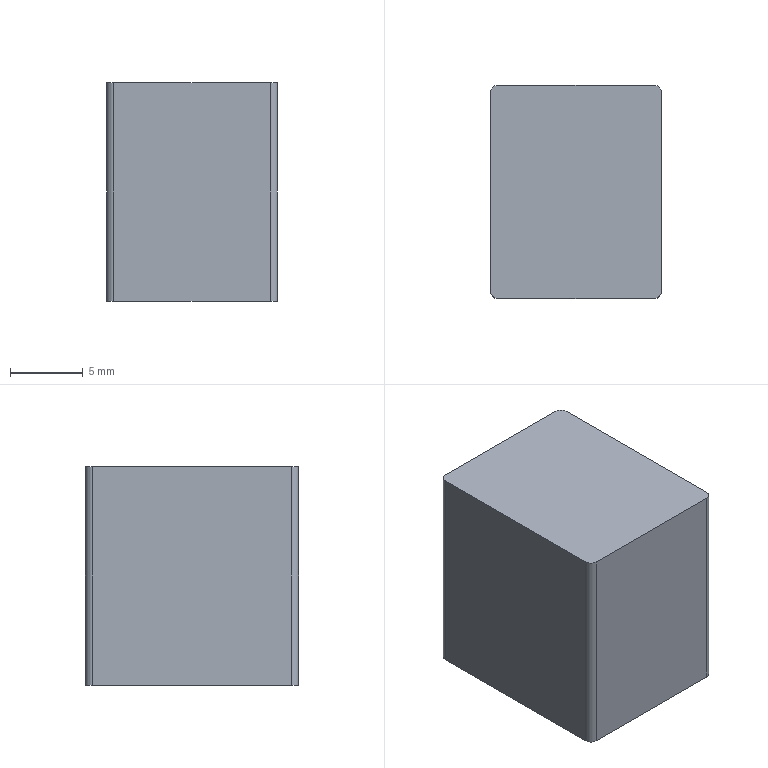Part | NX | features BREP 1 | 1 solid | 10 faces | box 11.7 x 14.6 x 15 mm | volume 2559 mm3 | plane 6 | cylinder 4 | commonest cylinder face diameters 1 x4
STEP:
#1=CARTESIAN_POINT('',(-5.35,7.3,-25.6));
#2=VERTEX_POINT('',#1);
#3=CARTESIAN_POINT('',(-5.85,6.8,-25.6));
#4=VERTEX_POINT('',#3);
#5=CARTESIAN_POINT('',(-5.35,6.8,-25.6));
#6=DIRECTION('',(0.,0.,1.));
#7=DIRECTION('',(1.,0.,0.));
#8=AXIS2_PLACEMENT_3D('',#5,#6,#7);
#9=CIRCLE('',#8,0.5);
#10=EDGE_CURVE('',#2,#4,#9,.T.);
#11=ORIENTED_EDGE('',*,*,#10,.F.);
#12=CARTESIAN_POINT('',(-5.35,7.3,-40.6));
#13=VERTEX_POINT('',#12);
#14=CARTESIAN_POINT('',(-5.35,7.3,-40.6));
#15=DIRECTION('',(0.,0.,1.));
#16=VECTOR('',#15,1000.);
#17=LINE('',#14,#16);
#18=EDGE_CURVE('',#13,#2,#17,.T.);
#19=ORIENTED_EDGE('',*,*,#18,.F.);
#20=CARTESIAN_POINT('',(-5.85,6.8,-40.6));
#21=VERTEX_POINT('',#20);
#22=CARTESIAN_POINT('',(-5.35,6.8,-40.6));
#23=DIRECTION('',(0.,0.,1.));
#24=DIRECTION('',(1.,0.,0.));
#25=AXIS2_PLACEMENT_3D('',#22,#23,#24);
#26=CIRCLE('',#25,0.5);
#27=EDGE_CURVE('',#13,#21,#26,.T.);
#28=ORIENTED_EDGE('',*,*,#27,.T.);
#29=CARTESIAN_POINT('',(-5.85,6.8,-40.6));
#30=DIRECTION('',(0.,0.,1.));
#31=VECTOR('',#30,1000.);
#32=LINE('',#29,#31);
#33=EDGE_CURVE('',#21,#4,#32,.T.);
#34=ORIENTED_EDGE('',*,*,#33,.T.);
#35=EDGE_LOOP('',(#11,#19,#28,#34));
#36=FACE_BOUND('',#35,.T.);
#37=CARTESIAN_POINT('',(-5.35,6.8,-40.6));
#38=DIRECTION('',(0.,0.,1.));
#39=DIRECTION('',(-1.,0.,0.));
#40=AXIS2_PLACEMENT_3D('',#37,#38,#39);
#41=CYLINDRICAL_SURFACE('',#40,0.5);
#42=ADVANCED_FACE('',(#36),#41,.T.);
#43=CARTESIAN_POINT('',(-5.85,-6.8,-25.6));
#44=VERTEX_POINT('',#43);
#45=CARTESIAN_POINT('',(-5.85,-6.8,-25.6));
#46=DIRECTION('',(0.,1.,0.));
#47=VECTOR('',#46,1000.);
#48=LINE('',#45,#47);
#49=EDGE_CURVE('',#44,#4,#48,.T.);
#50=ORIENTED_EDGE('',*,*,#49,.T.);
#51=ORIENTED_EDGE('',*,*,#33,.F.);
#52=CARTESIAN_POINT('',(-5.85,-6.8,-40.6));
#53=VERTEX_POINT('',#52);
#54=CARTESIAN_POINT('',(-5.85,-6.8,-40.6));
#55=DIRECTION('',(0.,1.,0.));
#56=VECTOR('',#55,1000.);
#57=LINE('',#54,#56);
#58=EDGE_CURVE('',#53,#21,#57,.T.);
#59=ORIENTED_EDGE('',*,*,#58,.F.);
#60=CARTESIAN_POINT('',(-5.85,-6.8,-40.6));
#61=DIRECTION('',(0.,0.,1.));
#62=VECTOR('',#61,1000.);
#63=LINE('',#60,#62);
#64=EDGE_CURVE('',#53,#44,#63,.T.);
#65=ORIENTED_EDGE('',*,*,#64,.T.);
#66=EDGE_LOOP('',(#50,#51,#59,#65));
#67=FACE_BOUND('',#66,.T.);
#68=CARTESIAN_POINT('',(-5.85,-6.8,-40.6));
#69=DIRECTION('',(1.,0.,0.));
#70=DIRECTION('',(0.,0.,1.));
#71=AXIS2_PLACEMENT_3D('',#68,#69,#70);
#72=PLANE('',#71);
#73=ADVANCED_FACE('',(#67),#72,.F.);
#74=CARTESIAN_POINT('',(-5.35,-7.3,-25.6));
#75=VERTEX_POINT('',#74);
#76=CARTESIAN_POINT('',(-5.35,-6.8,-25.6));
#77=DIRECTION('',(0.,0.,1.));
#78=DIRECTION('',(1.,0.,0.));
#79=AXIS2_PLACEMENT_3D('',#76,#77,#78);
#80=CIRCLE('',#79,0.5);
#81=EDGE_CURVE('',#44,#75,#80,.T.);
#82=ORIENTED_EDGE('',*,*,#81,.F.);
#83=ORIENTED_EDGE('',*,*,#64,.F.);
#84=CARTESIAN_POINT('',(-5.35,-7.3,-40.6));
#85=VERTEX_POINT('',#84);
#86=CARTESIAN_POINT('',(-5.35,-6.8,-40.6));
#87=DIRECTION('',(0.,0.,1.));
#88=DIRECTION('',(1.,0.,0.));
#89=AXIS2_PLACEMENT_3D('',#86,#87,#88);
#90=CIRCLE('',#89,0.5);
#91=EDGE_CURVE('',#53,#85,#90,.T.);
#92=ORIENTED_EDGE('',*,*,#91,.T.);
#93=CARTESIAN_POINT('',(-5.35,-7.3,-40.6));
#94=DIRECTION('',(0.,0.,1.));
#95=VECTOR('',#94,1000.);
#96=LINE('',#93,#95);
#97=EDGE_CURVE('',#85,#75,#96,.T.);
#98=ORIENTED_EDGE('',*,*,#97,.T.);
#99=EDGE_LOOP('',(#82,#83,#92,#98));
#100=FACE_BOUND('',#99,.T.);
#101=CARTESIAN_POINT('',(-5.35,-6.8,-40.6));
#102=DIRECTION('',(0.,0.,1.));
#103=DIRECTION('',(-1.,0.,0.));
#104=AXIS2_PLACEMENT_3D('',#101,#102,#103);
#105=CYLINDRICAL_SURFACE('',#104,0.5);
#106=ADVANCED_FACE('',(#100),#105,.T.);
#107=CARTESIAN_POINT('',(5.35,-7.3,-25.6));
#108=VERTEX_POINT('',#107);
#109=CARTESIAN_POINT('',(5.35,-7.3,-25.6));
#110=DIRECTION('',(-1.,0.,0.));
#111=VECTOR('',#110,1000.);
#112=LINE('',#109,#111);
#113=EDGE_CURVE('',#108,#75,#112,.T.);
#114=ORIENTED_EDGE('',*,*,#113,.T.);
#115=ORIENTED_EDGE('',*,*,#97,.F.);
#116=CARTESIAN_POINT('',(5.35,-7.3,-40.6));
#117=VERTEX_POINT('',#116);
#118=CARTESIAN_POINT('',(5.35,-7.3,-40.6));
#119=DIRECTION('',(-1.,0.,0.));
#120=VECTOR('',#119,1000.);
#121=LINE('',#118,#120);
#122=EDGE_CURVE('',#117,#85,#121,.T.);
#123=ORIENTED_EDGE('',*,*,#122,.F.);
#124=CARTESIAN_POINT('',(5.35,-7.3,-40.6));
#125=DIRECTION('',(0.,0.,1.));
#126=VECTOR('',#125,1000.);
#127=LINE('',#124,#126);
#128=EDGE_CURVE('',#117,#108,#127,.T.);
#129=ORIENTED_EDGE('',*,*,#128,.T.);
#130=EDGE_LOOP('',(#114,#115,#123,#129));
#131=FACE_BOUND('',#130,.T.);
#132=CARTESIAN_POINT('',(5.35,-7.3,-40.6));
#133=DIRECTION('',(0.,1.,0.));
#134=DIRECTION('',(1.,0.,0.));
#135=AXIS2_PLACEMENT_3D('',#132,#133,#134);
#136=PLANE('',#135);
#137=ADVANCED_FACE('',(#131),#136,.F.);
#138=CARTESIAN_POINT('',(5.85,-6.8,-25.6));
#139=VERTEX_POINT('',#138);
#140=CARTESIAN_POINT('',(5.35,-6.8,-25.6));
#141=DIRECTION('',(0.,0.,1.));
#142=DIRECTION('',(1.,0.,0.));
#143=AXIS2_PLACEMENT_3D('',#140,#141,#142);
#144=CIRCLE('',#143,0.5);
#145=EDGE_CURVE('',#108,#139,#144,.T.);
#146=ORIENTED_EDGE('',*,*,#145,.F.);
#147=ORIENTED_EDGE('',*,*,#128,.F.);
#148=CARTESIAN_POINT('',(5.85,-6.8,-40.6));
#149=VERTEX_POINT('',#148);
#150=CARTESIAN_POINT('',(5.35,-6.8,-40.6));
#151=DIRECTION('',(0.,0.,1.));
#152=DIRECTION('',(1.,0.,0.));
#153=AXIS2_PLACEMENT_3D('',#150,#151,#152);
#154=CIRCLE('',#153,0.5);
#155=EDGE_CURVE('',#117,#149,#154,.T.);
#156=ORIENTED_EDGE('',*,*,#155,.T.);
#157=CARTESIAN_POINT('',(5.85,-6.8,-40.6));
#158=DIRECTION('',(0.,0.,1.));
#159=VECTOR('',#158,1000.);
#160=LINE('',#157,#159);
#161=EDGE_CURVE('',#149,#139,#160,.T.);
#162=ORIENTED_EDGE('',*,*,#161,.T.);
#163=EDGE_LOOP('',(#146,#147,#156,#162));
#164=FACE_BOUND('',#163,.T.);
#165=CARTESIAN_POINT('',(5.35,-6.8,-40.6));
#166=DIRECTION('',(0.,0.,1.));
#167=DIRECTION('',(-1.,0.,0.));
#168=AXIS2_PLACEMENT_3D('',#165,#166,#167);
#169=CYLINDRICAL_SURFACE('',#168,0.5);
#170=ADVANCED_FACE('',(#164),#169,.T.);
#171=CARTESIAN_POINT('',(5.85,6.8,-25.6));
#172=VERTEX_POINT('',#171);
#173=CARTESIAN_POINT('',(5.85,6.8,-25.6));
#174=DIRECTION('',(0.,-1.,0.));
#175=VECTOR('',#174,1000.);
#176=LINE('',#173,#175);
#177=EDGE_CURVE('',#172,#139,#176,.T.);
#178=ORIENTED_EDGE('',*,*,#177,.T.);
#179=ORIENTED_EDGE('',*,*,#161,.F.);
#180=CARTESIAN_POINT('',(5.85,6.8,-40.6));
#181=VERTEX_POINT('',#180);
#182=CARTESIAN_POINT('',(5.85,6.8,-40.6));
#183=DIRECTION('',(0.,-1.,0.));
#184=VECTOR('',#183,1000.);
#185=LINE('',#182,#184);
#186=EDGE_CURVE('',#181,#149,#185,.T.);
#187=ORIENTED_EDGE('',*,*,#186,.F.);
#188=CARTESIAN_POINT('',(5.85,6.8,-40.6));
#189=DIRECTION('',(0.,0.,1.));
#190=VECTOR('',#189,1000.);
#191=LINE('',#188,#190);
#192=EDGE_CURVE('',#181,#172,#191,.T.);
#193=ORIENTED_EDGE('',*,*,#192,.T.);
#194=EDGE_LOOP('',(#178,#179,#187,#193));
#195=FACE_BOUND('',#194,.T.);
#196=CARTESIAN_POINT('',(5.85,6.8,-40.6));
#197=DIRECTION('',(-1.,0.,0.));
#198=DIRECTION('',(0.,0.,-1.));
#199=AXIS2_PLACEMENT_3D('',#196,#197,#198);
#200=PLANE('',#199);
#201=ADVANCED_FACE('',(#195),#200,.F.);
#202=CARTESIAN_POINT('',(5.35,7.3,-25.6));
#203=VERTEX_POINT('',#202);
#204=CARTESIAN_POINT('',(5.35,6.8,-25.6));
#205=DIRECTION('',(0.,0.,1.));
#206=DIRECTION('',(1.,0.,0.));
#207=AXIS2_PLACEMENT_3D('',#204,#205,#206);
#208=CIRCLE('',#207,0.5);
#209=EDGE_CURVE('',#172,#203,#208,.T.);
#210=ORIENTED_EDGE('',*,*,#209,.F.);
#211=ORIENTED_EDGE('',*,*,#192,.F.);
#212=CARTESIAN_POINT('',(5.35,7.3,-40.6));
#213=VERTEX_POINT('',#212);
#214=CARTESIAN_POINT('',(5.35,6.8,-40.6));
#215=DIRECTION('',(0.,0.,1.));
#216=DIRECTION('',(1.,0.,0.));
#217=AXIS2_PLACEMENT_3D('',#214,#215,#216);
#218=CIRCLE('',#217,0.5);
#219=EDGE_CURVE('',#181,#213,#218,.T.);
#220=ORIENTED_EDGE('',*,*,#219,.T.);
#221=CARTESIAN_POINT('',(5.35,7.3,-40.6));
#222=DIRECTION('',(0.,0.,1.));
#223=VECTOR('',#222,1000.);
#224=LINE('',#221,#223);
#225=EDGE_CURVE('',#213,#203,#224,.T.);
#226=ORIENTED_EDGE('',*,*,#225,.T.);
#227=EDGE_LOOP('',(#210,#211,#220,#226));
#228=FACE_BOUND('',#227,.T.);
#229=CARTESIAN_POINT('',(5.35,6.8,-40.6));
#230=DIRECTION('',(0.,0.,1.));
#231=DIRECTION('',(-1.,0.,0.));
#232=AXIS2_PLACEMENT_3D('',#229,#230,#231);
#233=CYLINDRICAL_SURFACE('',#232,0.5);
#234=ADVANCED_FACE('',(#228),#233,.T.);
#235=CARTESIAN_POINT('',(-5.35,7.3,-25.6));
#236=DIRECTION('',(1.,0.,0.));
#237=VECTOR('',#236,1000.);
#238=LINE('',#235,#237);
#239=EDGE_CURVE('',#2,#203,#238,.T.);
#240=ORIENTED_EDGE('',*,*,#239,.T.);
#241=ORIENTED_EDGE('',*,*,#225,.F.);
#242=CARTESIAN_POINT('',(-5.35,7.3,-40.6));
#243=DIRECTION('',(1.,0.,0.));
#244=VECTOR('',#243,1000.);
#245=LINE('',#242,#244);
#246=EDGE_CURVE('',#13,#213,#245,.T.);
#247=ORIENTED_EDGE('',*,*,#246,.F.);
#248=ORIENTED_EDGE('',*,*,#18,.T.);
#249=EDGE_LOOP('',(#240,#241,#247,#248));
#250=FACE_BOUND('',#249,.T.);
#251=CARTESIAN_POINT('',(-5.35,7.3,-40.6));
#252=DIRECTION('',(0.,-1.,0.));
#253=DIRECTION('',(0.,0.,1.));
#254=AXIS2_PLACEMENT_3D('',#251,#252,#253);
#255=PLANE('',#254);
#256=ADVANCED_FACE('',(#250),#255,.F.);
#257=ORIENTED_EDGE('',*,*,#27,.F.);
#258=ORIENTED_EDGE('',*,*,#246,.T.);
#259=ORIENTED_EDGE('',*,*,#219,.F.);
#260=ORIENTED_EDGE('',*,*,#186,.T.);
#261=ORIENTED_EDGE('',*,*,#155,.F.);
#262=ORIENTED_EDGE('',*,*,#122,.T.);
#263=ORIENTED_EDGE('',*,*,#91,.F.);
#264=ORIENTED_EDGE('',*,*,#58,.T.);
#265=EDGE_LOOP('',(#257,#258,#259,#260,#261,#262,#263,#264));
#266=FACE_BOUND('',#265,.T.);
#267=CARTESIAN_POINT('',(-5.35,6.8,-40.6));
#268=DIRECTION('',(0.,0.,1.));
#269=DIRECTION('',(-1.,0.,0.));
#270=AXIS2_PLACEMENT_3D('',#267,#268,#269);
#271=PLANE('',#270);
#272=ADVANCED_FACE('',(#266),#271,.F.);
#273=ORIENTED_EDGE('',*,*,#10,.T.);
#274=ORIENTED_EDGE('',*,*,#49,.F.);
#275=ORIENTED_EDGE('',*,*,#81,.T.);
#276=ORIENTED_EDGE('',*,*,#113,.F.);
#277=ORIENTED_EDGE('',*,*,#145,.T.);
#278=ORIENTED_EDGE('',*,*,#177,.F.);
#279=ORIENTED_EDGE('',*,*,#209,.T.);
#280=ORIENTED_EDGE('',*,*,#239,.F.);
#281=EDGE_LOOP('',(#273,#274,#275,#276,#277,#278,#279,#280));
#282=FACE_BOUND('',#281,.T.);
#283=CARTESIAN_POINT('',(-5.35,6.8,-25.6));
#284=DIRECTION('',(0.,0.,1.));
#285=DIRECTION('',(-1.,0.,0.));
#286=AXIS2_PLACEMENT_3D('',#283,#284,#285);
#287=PLANE('',#286);
#288=ADVANCED_FACE('',(#282),#287,.T.);
#289=CLOSED_SHELL('',(#42,#73,#106,#137,#170,#201,#234,#256,#272,#288));
#290=MANIFOLD_SOLID_BREP('',#289);
#291=(LENGTH_UNIT()NAMED_UNIT(*)SI_UNIT(.MILLI.,.METRE.));
#292=UNCERTAINTY_MEASURE_WITH_UNIT(LENGTH_MEASURE(0.00001),#291,'','');
#293=(NAMED_UNIT(*)PLANE_ANGLE_UNIT()SI_UNIT($,.RADIAN.));
#294=(NAMED_UNIT(*)SI_UNIT($,.STERADIAN.)SOLID_ANGLE_UNIT());
#295=(GEOMETRIC_REPRESENTATION_CONTEXT(3)GLOBAL_UNCERTAINTY_ASSIGNED_CONTEXT((#292))GLOBAL_UNIT_ASSIGNED_CONTEXT((#291,#293,#294))REPRESENTATION_CONTEXT('',''));
#296=ADVANCED_BREP_SHAPE_REPRESENTATION('',(#290),#295);